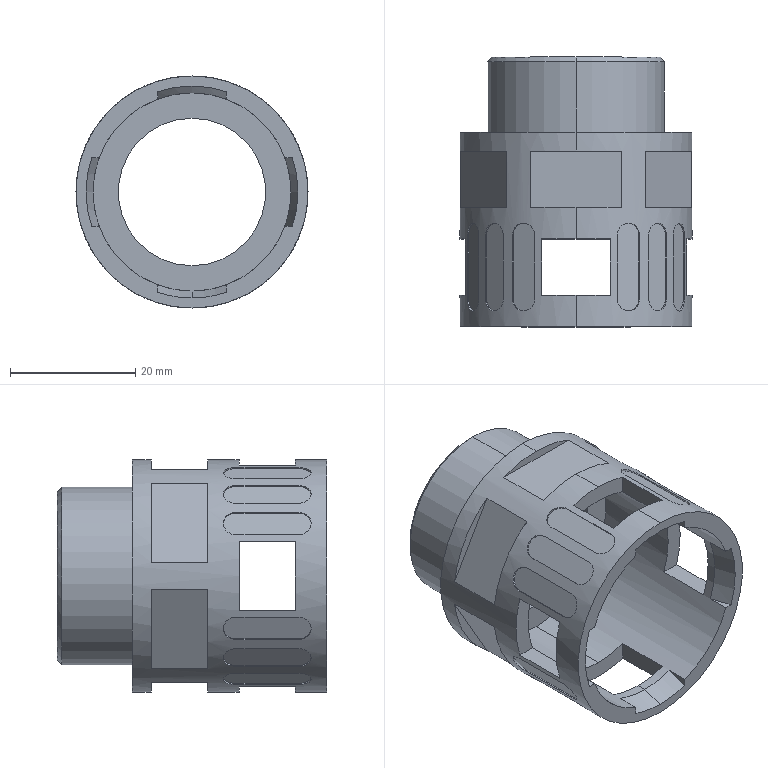Part | STEP file | PN_0001 part X2_00DC_X0 throw | 1 solid | 121 faces | box 37 x 43 x 37 mm | volume 10248 mm3 | plane 82 | cylinder 32 | cone 7 | commonest cylinder face diameters 4 x24 23.5 x2 28.3 x2 31.6 x2 37 x2